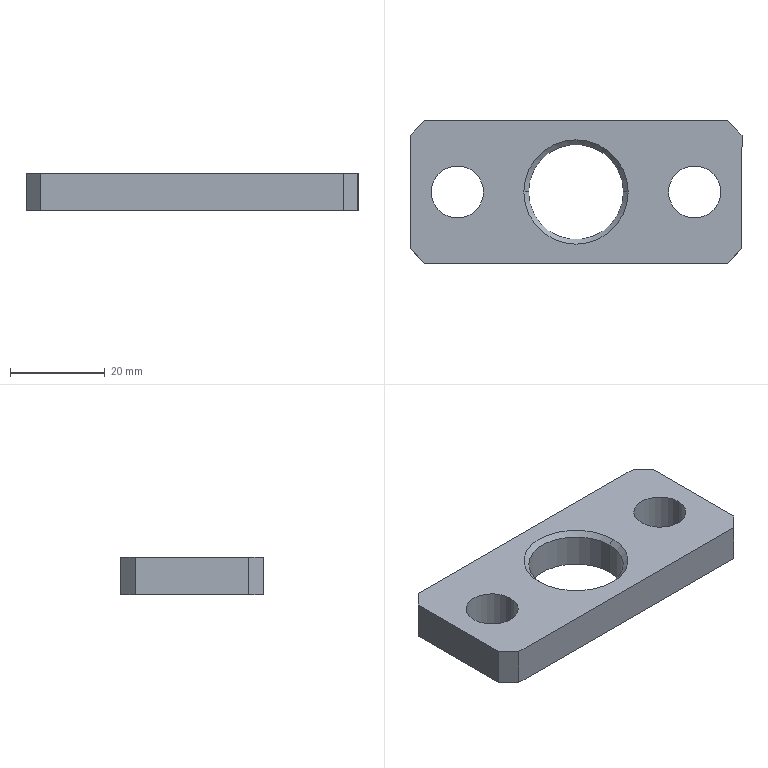Part | SolidWorks | features Chamfer 2, FlatPattern 1, ICE 1, SMBaseFlange 1, SheetMetal 1 | 1 solid | 18 faces | box 70 x 30 x 8 mm | volume 12590 mm3 | plane 10 | cylinder 6 | cone 2 | commonest cylinder face diameters 11 x4 20 x2
STEP:
#1=CARTESIAN_POINT('',(-10.,0.,-1.));
#2=VERTEX_POINT('',#1);
#3=CARTESIAN_POINT('',(10.,0.,-1.));
#4=VERTEX_POINT('',#3);
#5=CARTESIAN_POINT('',(0.,0.,-1.));
#6=DIRECTION('',(0.,0.,1.));
#7=DIRECTION('',(1.,0.,0.));
#8=AXIS2_PLACEMENT_3D('',#5,#6,#7);
#9=CIRCLE('',#8,10.);
#10=EDGE_CURVE('',#2,#4,#9,.T.);
#11=ORIENTED_EDGE('',*,*,#10,.F.);
#12=CARTESIAN_POINT('',(-11.,0.,0.));
#13=VERTEX_POINT('',#12);
#14=CARTESIAN_POINT('',(-10.,0.,-1.));
#15=DIRECTION('',(-0.7071,0.,0.7071));
#16=VECTOR('',#15,1000.);
#17=LINE('',#14,#16);
#18=EDGE_CURVE('',#2,#13,#17,.T.);
#19=ORIENTED_EDGE('',*,*,#18,.T.);
#20=CARTESIAN_POINT('',(11.,0.,0.));
#21=VERTEX_POINT('',#20);
#22=CARTESIAN_POINT('',(0.,0.,0.));
#23=DIRECTION('',(0.,0.,-1.));
#24=DIRECTION('',(1.,0.,0.));
#25=AXIS2_PLACEMENT_3D('',#22,#23,#24);
#26=CIRCLE('',#25,11.);
#27=EDGE_CURVE('',#21,#13,#26,.T.);
#28=ORIENTED_EDGE('',*,*,#27,.F.);
#29=CARTESIAN_POINT('',(10.,0.,-1.));
#30=DIRECTION('',(0.7071,0.,0.7071));
#31=VECTOR('',#30,1000.);
#32=LINE('',#29,#31);
#33=EDGE_CURVE('',#4,#21,#32,.T.);
#34=ORIENTED_EDGE('',*,*,#33,.F.);
#35=EDGE_LOOP('',(#11,#19,#28,#34));
#36=FACE_OUTER_BOUND('',#35,.T.);
#37=CARTESIAN_POINT('',(0.,0.,-1.));
#38=DIRECTION('',(0.,0.,1.));
#39=DIRECTION('',(1.,0.,0.));
#40=AXIS2_PLACEMENT_3D('',#37,#38,#39);
#41=CONICAL_SURFACE('',#40,10.,0.7854);
#42=ADVANCED_FACE('',(#36),#41,.F.);
#43=CARTESIAN_POINT('',(-10.,0.,-8.));
#44=VERTEX_POINT('',#43);
#45=CARTESIAN_POINT('',(10.,0.,-8.));
#46=VERTEX_POINT('',#45);
#47=CARTESIAN_POINT('',(0.,0.,-8.));
#48=DIRECTION('',(0.,0.,1.));
#49=DIRECTION('',(1.,0.,0.));
#50=AXIS2_PLACEMENT_3D('',#47,#48,#49);
#51=CIRCLE('',#50,10.);
#52=EDGE_CURVE('',#44,#46,#51,.T.);
#53=ORIENTED_EDGE('',*,*,#52,.F.);
#54=CARTESIAN_POINT('',(-10.,0.,-10.));
#55=DIRECTION('',(0.,0.,1.));
#56=VECTOR('',#55,1000.);
#57=LINE('',#54,#56);
#58=EDGE_CURVE('',#44,#2,#57,.T.);
#59=ORIENTED_EDGE('',*,*,#58,.T.);
#60=ORIENTED_EDGE('',*,*,#10,.T.);
#61=CARTESIAN_POINT('',(10.,0.,-10.));
#62=DIRECTION('',(0.,0.,1.));
#63=VECTOR('',#62,1000.);
#64=LINE('',#61,#63);
#65=EDGE_CURVE('',#46,#4,#64,.T.);
#66=ORIENTED_EDGE('',*,*,#65,.F.);
#67=EDGE_LOOP('',(#53,#59,#60,#66));
#68=FACE_OUTER_BOUND('',#67,.T.);
#69=CARTESIAN_POINT('',(0.,0.,-10.));
#70=DIRECTION('',(0.,0.,1.));
#71=DIRECTION('',(1.,0.,0.));
#72=AXIS2_PLACEMENT_3D('',#69,#70,#71);
#73=CYLINDRICAL_SURFACE('',#72,10.);
#74=ADVANCED_FACE('',(#68),#73,.F.);
#75=CARTESIAN_POINT('',(-30.5,0.,-8.));
#76=VERTEX_POINT('',#75);
#77=CARTESIAN_POINT('',(-19.5,0.,-8.));
#78=VERTEX_POINT('',#77);
#79=CARTESIAN_POINT('',(-25.,0.,-8.));
#80=DIRECTION('',(0.,0.,1.));
#81=DIRECTION('',(-1.,0.,0.));
#82=AXIS2_PLACEMENT_3D('',#79,#80,#81);
#83=CIRCLE('',#82,5.5);
#84=EDGE_CURVE('',#76,#78,#83,.T.);
#85=ORIENTED_EDGE('',*,*,#84,.F.);
#86=CARTESIAN_POINT('',(-30.5,0.,0.));
#87=VERTEX_POINT('',#86);
#88=CARTESIAN_POINT('',(-30.5,0.,-8.));
#89=DIRECTION('',(0.,0.,1.));
#90=VECTOR('',#89,1000.);
#91=LINE('',#88,#90);
#92=EDGE_CURVE('',#76,#87,#91,.T.);
#93=ORIENTED_EDGE('',*,*,#92,.T.);
#94=CARTESIAN_POINT('',(-19.5,0.,0.));
#95=VERTEX_POINT('',#94);
#96=CARTESIAN_POINT('',(-25.,0.,0.));
#97=DIRECTION('',(0.,0.,1.));
#98=DIRECTION('',(-1.,0.,0.));
#99=AXIS2_PLACEMENT_3D('',#96,#97,#98);
#100=CIRCLE('',#99,5.5);
#101=EDGE_CURVE('',#87,#95,#100,.T.);
#102=ORIENTED_EDGE('',*,*,#101,.T.);
#103=CARTESIAN_POINT('',(-19.5,0.,-8.));
#104=DIRECTION('',(0.,0.,1.));
#105=VECTOR('',#104,1000.);
#106=LINE('',#103,#105);
#107=EDGE_CURVE('',#78,#95,#106,.T.);
#108=ORIENTED_EDGE('',*,*,#107,.F.);
#109=EDGE_LOOP('',(#85,#93,#102,#108));
#110=FACE_OUTER_BOUND('',#109,.T.);
#111=CARTESIAN_POINT('',(-25.,0.,-8.));
#112=DIRECTION('',(0.,0.,1.));
#113=DIRECTION('',(1.,0.,0.));
#114=AXIS2_PLACEMENT_3D('',#111,#112,#113);
#115=CYLINDRICAL_SURFACE('',#114,5.5);
#116=ADVANCED_FACE('',(#110),#115,.F.);
#117=CARTESIAN_POINT('',(19.5,0.,-8.));
#118=VERTEX_POINT('',#117);
#119=CARTESIAN_POINT('',(30.5,0.,-8.));
#120=VERTEX_POINT('',#119);
#121=CARTESIAN_POINT('',(25.,0.,-8.));
#122=DIRECTION('',(0.,0.,1.));
#123=DIRECTION('',(1.,0.,0.));
#124=AXIS2_PLACEMENT_3D('',#121,#122,#123);
#125=CIRCLE('',#124,5.5);
#126=EDGE_CURVE('',#118,#120,#125,.T.);
#127=ORIENTED_EDGE('',*,*,#126,.F.);
#128=CARTESIAN_POINT('',(19.5,0.,0.));
#129=VERTEX_POINT('',#128);
#130=CARTESIAN_POINT('',(19.5,0.,-8.));
#131=DIRECTION('',(0.,0.,1.));
#132=VECTOR('',#131,1000.);
#133=LINE('',#130,#132);
#134=EDGE_CURVE('',#118,#129,#133,.T.);
#135=ORIENTED_EDGE('',*,*,#134,.T.);
#136=CARTESIAN_POINT('',(30.5,0.,0.));
#137=VERTEX_POINT('',#136);
#138=CARTESIAN_POINT('',(25.,0.,0.));
#139=DIRECTION('',(0.,0.,1.));
#140=DIRECTION('',(1.,0.,0.));
#141=AXIS2_PLACEMENT_3D('',#138,#139,#140);
#142=CIRCLE('',#141,5.5);
#143=EDGE_CURVE('',#129,#137,#142,.T.);
#144=ORIENTED_EDGE('',*,*,#143,.T.);
#145=CARTESIAN_POINT('',(30.5,0.,-8.));
#146=DIRECTION('',(0.,0.,1.));
#147=VECTOR('',#146,1000.);
#148=LINE('',#145,#147);
#149=EDGE_CURVE('',#120,#137,#148,.T.);
#150=ORIENTED_EDGE('',*,*,#149,.F.);
#151=EDGE_LOOP('',(#127,#135,#144,#150));
#152=FACE_OUTER_BOUND('',#151,.T.);
#153=CARTESIAN_POINT('',(25.,0.,-8.));
#154=DIRECTION('',(0.,0.,1.));
#155=DIRECTION('',(1.,0.,0.));
#156=AXIS2_PLACEMENT_3D('',#153,#154,#155);
#157=CYLINDRICAL_SURFACE('',#156,5.5);
#158=ADVANCED_FACE('',(#152),#157,.F.);
#159=CARTESIAN_POINT('',(-35.,12.,-8.));
#160=VERTEX_POINT('',#159);
#161=CARTESIAN_POINT('',(-35.,-12.,-8.));
#162=VERTEX_POINT('',#161);
#163=CARTESIAN_POINT('',(-35.,15.,-8.));
#164=DIRECTION('',(0.,-1.,0.));
#165=VECTOR('',#164,1000.);
#166=LINE('',#163,#165);
#167=EDGE_CURVE('',#160,#162,#166,.T.);
#168=ORIENTED_EDGE('',*,*,#167,.T.);
#169=CARTESIAN_POINT('',(-35.,-12.,0.));
#170=VERTEX_POINT('',#169);
#171=CARTESIAN_POINT('',(-35.,-12.,-8.));
#172=DIRECTION('',(0.,0.,1.));
#173=VECTOR('',#172,1000.);
#174=LINE('',#171,#173);
#175=EDGE_CURVE('',#162,#170,#174,.T.);
#176=ORIENTED_EDGE('',*,*,#175,.T.);
#177=CARTESIAN_POINT('',(-35.,12.,0.));
#178=VERTEX_POINT('',#177);
#179=CARTESIAN_POINT('',(-35.,15.,0.));
#180=DIRECTION('',(0.,-1.,0.));
#181=VECTOR('',#180,1000.);
#182=LINE('',#179,#181);
#183=EDGE_CURVE('',#178,#170,#182,.T.);
#184=ORIENTED_EDGE('',*,*,#183,.F.);
#185=CARTESIAN_POINT('',(-35.,12.,-8.));
#186=DIRECTION('',(0.,0.,-1.));
#187=VECTOR('',#186,1000.);
#188=LINE('',#185,#187);
#189=EDGE_CURVE('',#178,#160,#188,.T.);
#190=ORIENTED_EDGE('',*,*,#189,.T.);
#191=EDGE_LOOP('',(#168,#176,#184,#190));
#192=FACE_OUTER_BOUND('',#191,.T.);
#193=CARTESIAN_POINT('',(-35.,15.,-8.));
#194=DIRECTION('',(-1.,0.,0.));
#195=DIRECTION('',(0.,0.,1.));
#196=AXIS2_PLACEMENT_3D('',#193,#194,#195);
#197=PLANE('',#196);
#198=ADVANCED_FACE('',(#192),#197,.T.);
#199=CARTESIAN_POINT('',(32.,15.,0.));
#200=VERTEX_POINT('',#199);
#201=CARTESIAN_POINT('',(-32.,15.,0.));
#202=VERTEX_POINT('',#201);
#203=CARTESIAN_POINT('',(-35.,15.,0.));
#204=DIRECTION('',(-1.,0.,0.));
#205=VECTOR('',#204,1000.);
#206=LINE('',#203,#205);
#207=EDGE_CURVE('',#200,#202,#206,.T.);
#208=ORIENTED_EDGE('',*,*,#207,.F.);
#209=CARTESIAN_POINT('',(32.,15.,-8.));
#210=VERTEX_POINT('',#209);
#211=CARTESIAN_POINT('',(32.,15.,-8.));
#212=DIRECTION('',(0.,0.,-1.));
#213=VECTOR('',#212,1000.);
#214=LINE('',#211,#213);
#215=EDGE_CURVE('',#200,#210,#214,.T.);
#216=ORIENTED_EDGE('',*,*,#215,.T.);
#217=CARTESIAN_POINT('',(-32.,15.,-8.));
#218=VERTEX_POINT('',#217);
#219=CARTESIAN_POINT('',(-35.,15.,-8.));
#220=DIRECTION('',(-1.,0.,0.));
#221=VECTOR('',#220,1000.);
#222=LINE('',#219,#221);
#223=EDGE_CURVE('',#210,#218,#222,.T.);
#224=ORIENTED_EDGE('',*,*,#223,.T.);
#225=CARTESIAN_POINT('',(-32.,15.,-8.));
#226=DIRECTION('',(0.,0.,1.));
#227=VECTOR('',#226,1000.);
#228=LINE('',#225,#227);
#229=EDGE_CURVE('',#218,#202,#228,.T.);
#230=ORIENTED_EDGE('',*,*,#229,.T.);
#231=EDGE_LOOP('',(#208,#216,#224,#230));
#232=FACE_OUTER_BOUND('',#231,.T.);
#233=CARTESIAN_POINT('',(-35.,15.,-8.));
#234=DIRECTION('',(0.,1.,0.));
#235=DIRECTION('',(0.,0.,1.));
#236=AXIS2_PLACEMENT_3D('',#233,#234,#235);
#237=PLANE('',#236);
#238=ADVANCED_FACE('',(#232),#237,.T.);
#239=CARTESIAN_POINT('',(35.,-12.,-8.));
#240=VERTEX_POINT('',#239);
#241=CARTESIAN_POINT('',(35.,12.,-8.));
#242=VERTEX_POINT('',#241);
#243=CARTESIAN_POINT('',(35.,15.,-8.));
#244=DIRECTION('',(0.,1.,0.));
#245=VECTOR('',#244,1000.);
#246=LINE('',#243,#245);
#247=EDGE_CURVE('',#240,#242,#246,.T.);
#248=ORIENTED_EDGE('',*,*,#247,.T.);
#249=CARTESIAN_POINT('',(35.,12.,0.));
#250=VERTEX_POINT('',#249);
#251=CARTESIAN_POINT('',(35.,12.,-8.));
#252=DIRECTION('',(0.,0.,1.));
#253=VECTOR('',#252,1000.);
#254=LINE('',#251,#253);
#255=EDGE_CURVE('',#242,#250,#254,.T.);
#256=ORIENTED_EDGE('',*,*,#255,.T.);
#257=CARTESIAN_POINT('',(35.,-12.,0.));
#258=VERTEX_POINT('',#257);
#259=CARTESIAN_POINT('',(35.,15.,0.));
#260=DIRECTION('',(0.,1.,0.));
#261=VECTOR('',#260,1000.);
#262=LINE('',#259,#261);
#263=EDGE_CURVE('',#258,#250,#262,.T.);
#264=ORIENTED_EDGE('',*,*,#263,.F.);
#265=CARTESIAN_POINT('',(35.,-12.,-8.));
#266=DIRECTION('',(0.,0.,-1.));
#267=VECTOR('',#266,1000.);
#268=LINE('',#265,#267);
#269=EDGE_CURVE('',#258,#240,#268,.T.);
#270=ORIENTED_EDGE('',*,*,#269,.T.);
#271=EDGE_LOOP('',(#248,#256,#264,#270));
#272=FACE_OUTER_BOUND('',#271,.T.);
#273=CARTESIAN_POINT('',(35.,15.,-8.));
#274=DIRECTION('',(1.,0.,0.));
#275=DIRECTION('',(0.,0.,-1.));
#276=AXIS2_PLACEMENT_3D('',#273,#274,#275);
#277=PLANE('',#276);
#278=ADVANCED_FACE('',(#272),#277,.T.);
#279=CARTESIAN_POINT('',(-32.,-15.,-8.));
#280=VERTEX_POINT('',#279);
#281=CARTESIAN_POINT('',(32.,-15.,-8.));
#282=VERTEX_POINT('',#281);
#283=CARTESIAN_POINT('',(-35.,-15.,-8.));
#284=DIRECTION('',(1.,0.,0.));
#285=VECTOR('',#284,1000.);
#286=LINE('',#283,#285);
#287=EDGE_CURVE('',#280,#282,#286,.T.);
#288=ORIENTED_EDGE('',*,*,#287,.T.);
#289=CARTESIAN_POINT('',(32.,-15.,0.));
#290=VERTEX_POINT('',#289);
#291=CARTESIAN_POINT('',(32.,-15.,-8.));
#292=DIRECTION('',(0.,0.,1.));
#293=VECTOR('',#292,1000.);
#294=LINE('',#291,#293);
#295=EDGE_CURVE('',#282,#290,#294,.T.);
#296=ORIENTED_EDGE('',*,*,#295,.T.);
#297=CARTESIAN_POINT('',(-32.,-15.,0.));
#298=VERTEX_POINT('',#297);
#299=CARTESIAN_POINT('',(-35.,-15.,0.));
#300=DIRECTION('',(1.,0.,0.));
#301=VECTOR('',#300,1000.);
#302=LINE('',#299,#301);
#303=EDGE_CURVE('',#298,#290,#302,.T.);
#304=ORIENTED_EDGE('',*,*,#303,.F.);
#305=CARTESIAN_POINT('',(-32.,-15.,-8.));
#306=DIRECTION('',(0.,0.,-1.));
#307=VECTOR('',#306,1000.);
#308=LINE('',#305,#307);
#309=EDGE_CURVE('',#298,#280,#308,.T.);
#310=ORIENTED_EDGE('',*,*,#309,.T.);
#311=EDGE_LOOP('',(#288,#296,#304,#310));
#312=FACE_OUTER_BOUND('',#311,.T.);
#313=CARTESIAN_POINT('',(-35.,-15.,-8.));
#314=DIRECTION('',(0.,-1.,0.));
#315=DIRECTION('',(0.,0.,-1.));
#316=AXIS2_PLACEMENT_3D('',#313,#314,#315);
#317=PLANE('',#316);
#318=ADVANCED_FACE('',(#312),#317,.T.);
#319=CARTESIAN_POINT('',(0.,0.,-8.));
#320=DIRECTION('',(0.,0.,1.));
#321=DIRECTION('',(1.,0.,0.));
#322=AXIS2_PLACEMENT_3D('',#319,#320,#321);
#323=CIRCLE('',#322,10.);
#324=EDGE_CURVE('',#46,#44,#323,.T.);
#325=ORIENTED_EDGE('',*,*,#324,.T.);
#326=ORIENTED_EDGE('',*,*,#52,.T.);
#327=EDGE_LOOP('',(#325,#326));
#328=FACE_BOUND('',#327,.T.);
#329=CARTESIAN_POINT('',(-25.,0.,-8.));
#330=DIRECTION('',(0.,0.,1.));
#331=DIRECTION('',(-1.,0.,0.));
#332=AXIS2_PLACEMENT_3D('',#329,#330,#331);
#333=CIRCLE('',#332,5.5);
#334=EDGE_CURVE('',#78,#76,#333,.T.);
#335=ORIENTED_EDGE('',*,*,#334,.T.);
#336=ORIENTED_EDGE('',*,*,#84,.T.);
#337=EDGE_LOOP('',(#335,#336));
#338=FACE_BOUND('',#337,.T.);
#339=CARTESIAN_POINT('',(25.,0.,-8.));
#340=DIRECTION('',(0.,0.,1.));
#341=DIRECTION('',(1.,0.,0.));
#342=AXIS2_PLACEMENT_3D('',#339,#340,#341);
#343=CIRCLE('',#342,5.5);
#344=EDGE_CURVE('',#120,#118,#343,.T.);
#345=ORIENTED_EDGE('',*,*,#344,.T.);
#346=ORIENTED_EDGE('',*,*,#126,.T.);
#347=EDGE_LOOP('',(#345,#346));
#348=FACE_BOUND('',#347,.T.);
#349=ORIENTED_EDGE('',*,*,#223,.F.);
#350=CARTESIAN_POINT('',(35.,12.,-8.));
#351=DIRECTION('',(0.7071,-0.7071,0.));
#352=VECTOR('',#351,1000.);
#353=LINE('',#350,#352);
#354=EDGE_CURVE('',#210,#242,#353,.T.);
#355=ORIENTED_EDGE('',*,*,#354,.T.);
#356=ORIENTED_EDGE('',*,*,#247,.F.);
#357=CARTESIAN_POINT('',(32.,-15.,-8.));
#358=DIRECTION('',(-0.7071,-0.7071,0.));
#359=VECTOR('',#358,1000.);
#360=LINE('',#357,#359);
#361=EDGE_CURVE('',#240,#282,#360,.T.);
#362=ORIENTED_EDGE('',*,*,#361,.T.);
#363=ORIENTED_EDGE('',*,*,#287,.F.);
#364=CARTESIAN_POINT('',(-35.,-12.,-8.));
#365=DIRECTION('',(-0.7071,0.7071,0.));
#366=VECTOR('',#365,1000.);
#367=LINE('',#364,#366);
#368=EDGE_CURVE('',#280,#162,#367,.T.);
#369=ORIENTED_EDGE('',*,*,#368,.T.);
#370=ORIENTED_EDGE('',*,*,#167,.F.);
#371=CARTESIAN_POINT('',(-32.,15.,-8.));
#372=DIRECTION('',(0.7071,0.7071,0.));
#373=VECTOR('',#372,1000.);
#374=LINE('',#371,#373);
#375=EDGE_CURVE('',#160,#218,#374,.T.);
#376=ORIENTED_EDGE('',*,*,#375,.T.);
#377=EDGE_LOOP('',(#349,#355,#356,#362,#363,#369,#370,#376));
#378=FACE_OUTER_BOUND('',#377,.T.);
#379=CARTESIAN_POINT('',(0.,0.,-8.));
#380=DIRECTION('',(0.,0.,1.));
#381=DIRECTION('',(1.,0.,0.));
#382=AXIS2_PLACEMENT_3D('',#379,#380,#381);
#383=PLANE('',#382);
#384=ADVANCED_FACE('',(#328,#338,#348,#378),#383,.F.);
#385=ORIENTED_EDGE('',*,*,#27,.T.);
#386=CARTESIAN_POINT('',(0.,0.,0.));
#387=DIRECTION('',(0.,0.,-1.));
#388=DIRECTION('',(1.,0.,0.));
#389=AXIS2_PLACEMENT_3D('',#386,#387,#388);
#390=CIRCLE('',#389,11.);
#391=EDGE_CURVE('',#13,#21,#390,.T.);
#392=ORIENTED_EDGE('',*,*,#391,.T.);
#393=EDGE_LOOP('',(#385,#392));
#394=FACE_BOUND('',#393,.T.);
#395=CARTESIAN_POINT('',(-25.,0.,0.));
#396=DIRECTION('',(0.,0.,1.));
#397=DIRECTION('',(-1.,0.,0.));
#398=AXIS2_PLACEMENT_3D('',#395,#396,#397);
#399=CIRCLE('',#398,5.5);
#400=EDGE_CURVE('',#95,#87,#399,.T.);
#401=ORIENTED_EDGE('',*,*,#400,.F.);
#402=ORIENTED_EDGE('',*,*,#101,.F.);
#403=EDGE_LOOP('',(#401,#402));
#404=FACE_BOUND('',#403,.T.);
#405=CARTESIAN_POINT('',(25.,0.,0.));
#406=DIRECTION('',(0.,0.,1.));
#407=DIRECTION('',(1.,0.,0.));
#408=AXIS2_PLACEMENT_3D('',#405,#406,#407);
#409=CIRCLE('',#408,5.5);
#410=EDGE_CURVE('',#137,#129,#409,.T.);
#411=ORIENTED_EDGE('',*,*,#410,.F.);
#412=ORIENTED_EDGE('',*,*,#143,.F.);
#413=EDGE_LOOP('',(#411,#412));
#414=FACE_BOUND('',#413,.T.);
#415=ORIENTED_EDGE('',*,*,#263,.T.);
#416=CARTESIAN_POINT('',(23.5,23.5,0.));
#417=DIRECTION('',(-0.7071,0.7071,0.));
#418=VECTOR('',#417,1000.);
#419=LINE('',#416,#418);
#420=EDGE_CURVE('',#250,#200,#419,.T.);
#421=ORIENTED_EDGE('',*,*,#420,.T.);
#422=ORIENTED_EDGE('',*,*,#207,.T.);
#423=CARTESIAN_POINT('',(-23.5,23.5,0.));
#424=DIRECTION('',(-0.7071,-0.7071,0.));
#425=VECTOR('',#424,1000.);
#426=LINE('',#423,#425);
#427=EDGE_CURVE('',#202,#178,#426,.T.);
#428=ORIENTED_EDGE('',*,*,#427,.T.);
#429=ORIENTED_EDGE('',*,*,#183,.T.);
#430=CARTESIAN_POINT('',(-23.5,-23.5,0.));
#431=DIRECTION('',(0.7071,-0.7071,0.));
#432=VECTOR('',#431,1000.);
#433=LINE('',#430,#432);
#434=EDGE_CURVE('',#170,#298,#433,.T.);
#435=ORIENTED_EDGE('',*,*,#434,.T.);
#436=ORIENTED_EDGE('',*,*,#303,.T.);
#437=CARTESIAN_POINT('',(23.5,-23.5,0.));
#438=DIRECTION('',(0.7071,0.7071,0.));
#439=VECTOR('',#438,1000.);
#440=LINE('',#437,#439);
#441=EDGE_CURVE('',#290,#258,#440,.T.);
#442=ORIENTED_EDGE('',*,*,#441,.T.);
#443=EDGE_LOOP('',(#415,#421,#422,#428,#429,#435,#436,#442));
#444=FACE_OUTER_BOUND('',#443,.T.);
#445=CARTESIAN_POINT('',(0.,0.,0.));
#446=DIRECTION('',(0.,0.,1.));
#447=DIRECTION('',(1.,0.,0.));
#448=AXIS2_PLACEMENT_3D('',#445,#446,#447);
#449=PLANE('',#448);
#450=ADVANCED_FACE('',(#394,#404,#414,#444),#449,.T.);
#451=ORIENTED_EDGE('',*,*,#134,.F.);
#452=ORIENTED_EDGE('',*,*,#344,.F.);
#453=ORIENTED_EDGE('',*,*,#149,.T.);
#454=ORIENTED_EDGE('',*,*,#410,.T.);
#455=EDGE_LOOP('',(#451,#452,#453,#454));
#456=FACE_OUTER_BOUND('',#455,.T.);
#457=CARTESIAN_POINT('',(25.,0.,-8.));
#458=DIRECTION('',(0.,0.,1.));
#459=DIRECTION('',(1.,0.,0.));
#460=AXIS2_PLACEMENT_3D('',#457,#458,#459);
#461=CYLINDRICAL_SURFACE('',#460,5.5);
#462=ADVANCED_FACE('',(#456),#461,.F.);
#463=ORIENTED_EDGE('',*,*,#92,.F.);
#464=ORIENTED_EDGE('',*,*,#334,.F.);
#465=ORIENTED_EDGE('',*,*,#107,.T.);
#466=ORIENTED_EDGE('',*,*,#400,.T.);
#467=EDGE_LOOP('',(#463,#464,#465,#466));
#468=FACE_OUTER_BOUND('',#467,.T.);
#469=CARTESIAN_POINT('',(-25.,0.,-8.));
#470=DIRECTION('',(0.,0.,1.));
#471=DIRECTION('',(1.,0.,0.));
#472=AXIS2_PLACEMENT_3D('',#469,#470,#471);
#473=CYLINDRICAL_SURFACE('',#472,5.5);
#474=ADVANCED_FACE('',(#468),#473,.F.);
#475=ORIENTED_EDGE('',*,*,#354,.F.);
#476=ORIENTED_EDGE('',*,*,#215,.F.);
#477=ORIENTED_EDGE('',*,*,#420,.F.);
#478=ORIENTED_EDGE('',*,*,#255,.F.);
#479=EDGE_LOOP('',(#475,#476,#477,#478));
#480=FACE_OUTER_BOUND('',#479,.T.);
#481=CARTESIAN_POINT('',(35.,12.,-8.));
#482=DIRECTION('',(-0.7071,-0.7071,0.));
#483=DIRECTION('',(0.,0.,1.));
#484=AXIS2_PLACEMENT_3D('',#481,#482,#483);
#485=PLANE('',#484);
#486=ADVANCED_FACE('',(#480),#485,.F.);
#487=ORIENTED_EDGE('',*,*,#361,.F.);
#488=ORIENTED_EDGE('',*,*,#269,.F.);
#489=ORIENTED_EDGE('',*,*,#441,.F.);
#490=ORIENTED_EDGE('',*,*,#295,.F.);
#491=EDGE_LOOP('',(#487,#488,#489,#490));
#492=FACE_OUTER_BOUND('',#491,.T.);
#493=CARTESIAN_POINT('',(32.,-15.,-8.));
#494=DIRECTION('',(-0.7071,0.7071,0.));
#495=DIRECTION('',(0.,0.,1.));
#496=AXIS2_PLACEMENT_3D('',#493,#494,#495);
#497=PLANE('',#496);
#498=ADVANCED_FACE('',(#492),#497,.F.);
#499=ORIENTED_EDGE('',*,*,#368,.F.);
#500=ORIENTED_EDGE('',*,*,#309,.F.);
#501=ORIENTED_EDGE('',*,*,#434,.F.);
#502=ORIENTED_EDGE('',*,*,#175,.F.);
#503=EDGE_LOOP('',(#499,#500,#501,#502));
#504=FACE_OUTER_BOUND('',#503,.T.);
#505=CARTESIAN_POINT('',(-35.,-12.,-8.));
#506=DIRECTION('',(0.7071,0.7071,0.));
#507=DIRECTION('',(0.,0.,1.));
#508=AXIS2_PLACEMENT_3D('',#505,#506,#507);
#509=PLANE('',#508);
#510=ADVANCED_FACE('',(#504),#509,.F.);
#511=ORIENTED_EDGE('',*,*,#375,.F.);
#512=ORIENTED_EDGE('',*,*,#189,.F.);
#513=ORIENTED_EDGE('',*,*,#427,.F.);
#514=ORIENTED_EDGE('',*,*,#229,.F.);
#515=EDGE_LOOP('',(#511,#512,#513,#514));
#516=FACE_OUTER_BOUND('',#515,.T.);
#517=CARTESIAN_POINT('',(-32.,15.,-8.));
#518=DIRECTION('',(0.7071,-0.7071,0.));
#519=DIRECTION('',(0.,0.,1.));
#520=AXIS2_PLACEMENT_3D('',#517,#518,#519);
#521=PLANE('',#520);
#522=ADVANCED_FACE('',(#516),#521,.F.);
#523=ORIENTED_EDGE('',*,*,#58,.F.);
#524=ORIENTED_EDGE('',*,*,#324,.F.);
#525=ORIENTED_EDGE('',*,*,#65,.T.);
#526=CARTESIAN_POINT('',(0.,0.,-1.));
#527=DIRECTION('',(0.,0.,1.));
#528=DIRECTION('',(1.,0.,0.));
#529=AXIS2_PLACEMENT_3D('',#526,#527,#528);
#530=CIRCLE('',#529,10.);
#531=EDGE_CURVE('',#4,#2,#530,.T.);
#532=ORIENTED_EDGE('',*,*,#531,.T.);
#533=EDGE_LOOP('',(#523,#524,#525,#532));
#534=FACE_OUTER_BOUND('',#533,.T.);
#535=CARTESIAN_POINT('',(0.,0.,-10.));
#536=DIRECTION('',(0.,0.,1.));
#537=DIRECTION('',(1.,0.,0.));
#538=AXIS2_PLACEMENT_3D('',#535,#536,#537);
#539=CYLINDRICAL_SURFACE('',#538,10.);
#540=ADVANCED_FACE('',(#534),#539,.F.);
#541=ORIENTED_EDGE('',*,*,#18,.F.);
#542=ORIENTED_EDGE('',*,*,#531,.F.);
#543=ORIENTED_EDGE('',*,*,#33,.T.);
#544=ORIENTED_EDGE('',*,*,#391,.F.);
#545=EDGE_LOOP('',(#541,#542,#543,#544));
#546=FACE_OUTER_BOUND('',#545,.T.);
#547=CARTESIAN_POINT('',(0.,0.,-1.));
#548=DIRECTION('',(0.,0.,1.));
#549=DIRECTION('',(1.,0.,0.));
#550=AXIS2_PLACEMENT_3D('',#547,#548,#549);
#551=CONICAL_SURFACE('',#550,10.,0.7854);
#552=ADVANCED_FACE('',(#546),#551,.F.);
#553=CLOSED_SHELL('',(#42,#74,#116,#158,#198,#238,#278,#318,#384,#450,#462,#474,#486,#498,#510,#522,#540,#552));
#554=MANIFOLD_SOLID_BREP('',#553);
#555=CARTESIAN_POINT('',(0.,0.,0.));
#556=DIRECTION('',(0.,0.,1.));
#557=DIRECTION('',(1.,0.,0.));
#558=AXIS2_PLACEMENT_3D('',#555,#556,#557);
#559=(LENGTH_UNIT()NAMED_UNIT(*)SI_UNIT(.MILLI.,.METRE.));
#560=UNCERTAINTY_MEASURE_WITH_UNIT(LENGTH_MEASURE(0.00001),#559,'','');
#561=(NAMED_UNIT(*)PLANE_ANGLE_UNIT()SI_UNIT($,.RADIAN.));
#562=(NAMED_UNIT(*)SI_UNIT($,.STERADIAN.)SOLID_ANGLE_UNIT());
#563=(GEOMETRIC_REPRESENTATION_CONTEXT(3)GLOBAL_UNCERTAINTY_ASSIGNED_CONTEXT((#560))GLOBAL_UNIT_ASSIGNED_CONTEXT((#559,#561,#562))REPRESENTATION_CONTEXT('',''));
#564=ADVANCED_BREP_SHAPE_REPRESENTATION('',(#554,#558),#563);